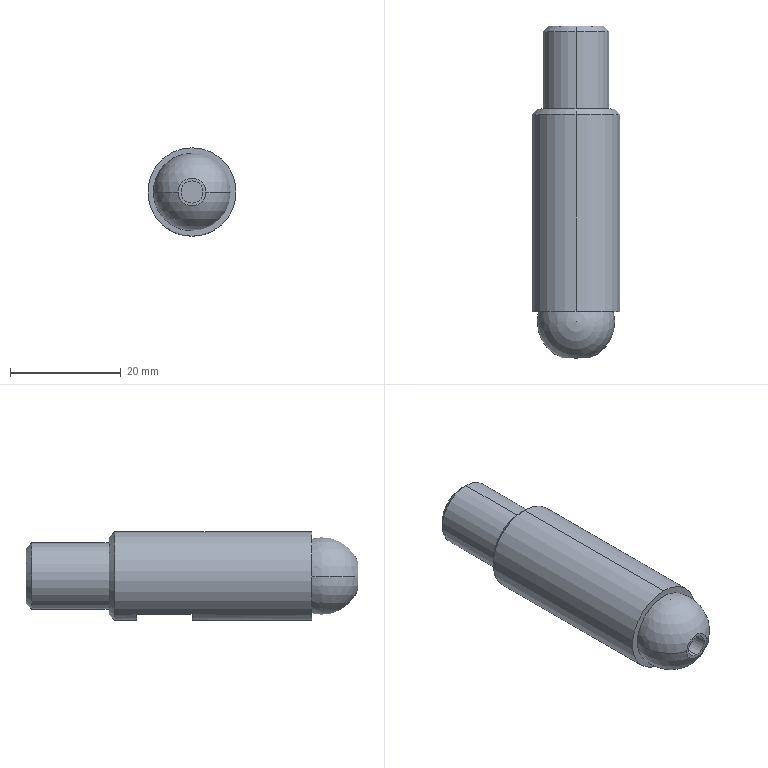Part | SolidWorks | features ICE 3, Chamfer 1, Revolution 1 | 1 solid | 24 faces | box 16 x 60 x 16 mm | volume 8216 mm3 | cylinder 9 | plane 9 | cone 4 | sphere 2 | commonest cylinder face diameters 12 x3 4 x2 8 x2 16 x2
STEP:
#1=CARTESIAN_POINT('',(0.,45.,7.));
#2=VERTEX_POINT('',#1);
#3=CARTESIAN_POINT('',(0.,45.,-7.));
#4=VERTEX_POINT('',#3);
#5=CARTESIAN_POINT('',(0.,45.,0.));
#6=DIRECTION('',(0.,1.,0.));
#7=DIRECTION('',(0.,0.,1.));
#8=AXIS2_PLACEMENT_3D('',#5,#6,#7);
#9=CIRCLE('',#8,7.);
#10=EDGE_CURVE('',#2,#4,#9,.T.);
#11=ORIENTED_EDGE('',*,*,#10,.F.);
#12=CARTESIAN_POINT('',(0.,44.,8.));
#13=VERTEX_POINT('',#12);
#14=CARTESIAN_POINT('',(0.,45.,7.));
#15=DIRECTION('',(0.,-0.7071,0.7071));
#16=VECTOR('',#15,1000.);
#17=LINE('',#14,#16);
#18=EDGE_CURVE('',#2,#13,#17,.T.);
#19=ORIENTED_EDGE('',*,*,#18,.T.);
#20=CARTESIAN_POINT('',(0.,44.,-8.));
#21=VERTEX_POINT('',#20);
#22=CARTESIAN_POINT('',(0.,44.,0.));
#23=DIRECTION('',(0.,-1.,0.));
#24=DIRECTION('',(0.,0.,1.));
#25=AXIS2_PLACEMENT_3D('',#22,#23,#24);
#26=CIRCLE('',#25,8.);
#27=EDGE_CURVE('',#21,#13,#26,.T.);
#28=ORIENTED_EDGE('',*,*,#27,.F.);
#29=CARTESIAN_POINT('',(0.,45.,-7.));
#30=DIRECTION('',(0.,-0.7071,-0.7071));
#31=VECTOR('',#30,1000.);
#32=LINE('',#29,#31);
#33=EDGE_CURVE('',#4,#21,#32,.T.);
#34=ORIENTED_EDGE('',*,*,#33,.F.);
#35=EDGE_LOOP('',(#11,#19,#28,#34));
#36=FACE_OUTER_BOUND('',#35,.T.);
#37=CARTESIAN_POINT('',(0.,45.,0.));
#38=DIRECTION('',(0.,-1.,0.));
#39=DIRECTION('',(0.,0.,-1.));
#40=AXIS2_PLACEMENT_3D('',#37,#38,#39);
#41=CONICAL_SURFACE('',#40,7.,0.7854);
#42=ADVANCED_FACE('',(#36),#41,.T.);
#43=CARTESIAN_POINT('',(0.,60.,5.));
#44=VERTEX_POINT('',#43);
#45=CARTESIAN_POINT('',(0.,60.,-5.));
#46=VERTEX_POINT('',#45);
#47=CARTESIAN_POINT('',(0.,60.,0.));
#48=DIRECTION('',(0.,1.,0.));
#49=DIRECTION('',(0.,0.,1.));
#50=AXIS2_PLACEMENT_3D('',#47,#48,#49);
#51=CIRCLE('',#50,5.);
#52=EDGE_CURVE('',#44,#46,#51,.T.);
#53=ORIENTED_EDGE('',*,*,#52,.F.);
#54=CARTESIAN_POINT('',(0.,59.,6.));
#55=VERTEX_POINT('',#54);
#56=CARTESIAN_POINT('',(0.,60.,5.));
#57=DIRECTION('',(0.,-0.7071,0.7071));
#58=VECTOR('',#57,1000.);
#59=LINE('',#56,#58);
#60=EDGE_CURVE('',#44,#55,#59,.T.);
#61=ORIENTED_EDGE('',*,*,#60,.T.);
#62=CARTESIAN_POINT('',(0.,59.,-6.));
#63=VERTEX_POINT('',#62);
#64=CARTESIAN_POINT('',(0.,59.,0.));
#65=DIRECTION('',(0.,-1.,0.));
#66=DIRECTION('',(0.,0.,1.));
#67=AXIS2_PLACEMENT_3D('',#64,#65,#66);
#68=CIRCLE('',#67,6.);
#69=EDGE_CURVE('',#63,#55,#68,.T.);
#70=ORIENTED_EDGE('',*,*,#69,.F.);
#71=CARTESIAN_POINT('',(0.,60.,-5.));
#72=DIRECTION('',(0.,-0.7071,-0.7071));
#73=VECTOR('',#72,1000.);
#74=LINE('',#71,#73);
#75=EDGE_CURVE('',#46,#63,#74,.T.);
#76=ORIENTED_EDGE('',*,*,#75,.F.);
#77=EDGE_LOOP('',(#53,#61,#70,#76));
#78=FACE_OUTER_BOUND('',#77,.T.);
#79=CARTESIAN_POINT('',(0.,60.,0.));
#80=DIRECTION('',(0.,-1.,0.));
#81=DIRECTION('',(0.,0.,-1.));
#82=AXIS2_PLACEMENT_3D('',#79,#80,#81);
#83=CONICAL_SURFACE('',#82,5.,0.7854);
#84=ADVANCED_FACE('',(#78),#83,.T.);
#85=ORIENTED_EDGE('',*,*,#69,.T.);
#86=CARTESIAN_POINT('',(0.,45.,6.));
#87=VERTEX_POINT('',#86);
#88=CARTESIAN_POINT('',(0.,60.,6.));
#89=DIRECTION('',(0.,-1.,0.));
#90=VECTOR('',#89,1000.);
#91=LINE('',#88,#90);
#92=EDGE_CURVE('',#55,#87,#91,.T.);
#93=ORIENTED_EDGE('',*,*,#92,.T.);
#94=CARTESIAN_POINT('',(0.,45.,-6.));
#95=VERTEX_POINT('',#94);
#96=CARTESIAN_POINT('',(0.,45.,0.));
#97=DIRECTION('',(0.,1.,0.));
#98=DIRECTION('',(0.,0.,1.));
#99=AXIS2_PLACEMENT_3D('',#96,#97,#98);
#100=CIRCLE('',#99,6.);
#101=EDGE_CURVE('',#87,#95,#100,.T.);
#102=ORIENTED_EDGE('',*,*,#101,.T.);
#103=CARTESIAN_POINT('',(0.,60.,-6.));
#104=DIRECTION('',(0.,-1.,0.));
#105=VECTOR('',#104,1000.);
#106=LINE('',#103,#105);
#107=EDGE_CURVE('',#63,#95,#106,.T.);
#108=ORIENTED_EDGE('',*,*,#107,.F.);
#109=EDGE_LOOP('',(#85,#93,#102,#108));
#110=FACE_OUTER_BOUND('',#109,.T.);
#111=CARTESIAN_POINT('',(0.,60.,0.));
#112=DIRECTION('',(0.,-1.,0.));
#113=DIRECTION('',(0.,0.,-1.));
#114=AXIS2_PLACEMENT_3D('',#111,#112,#113);
#115=CYLINDRICAL_SURFACE('',#114,6.);
#116=ADVANCED_FACE('',(#110),#115,.T.);
#117=ORIENTED_EDGE('',*,*,#27,.T.);
#118=CARTESIAN_POINT('',(0.,8.392,8.));
#119=VERTEX_POINT('',#118);
#120=CARTESIAN_POINT('',(0.,0.,8.));
#121=DIRECTION('',(0.,-1.,0.));
#122=VECTOR('',#121,1000.);
#123=LINE('',#120,#122);
#124=EDGE_CURVE('',#13,#119,#123,.T.);
#125=ORIENTED_EDGE('',*,*,#124,.T.);
#126=CARTESIAN_POINT('',(0.,8.392,-8.));
#127=VERTEX_POINT('',#126);
#128=CARTESIAN_POINT('',(0.,8.392,0.));
#129=DIRECTION('',(0.,-1.,0.));
#130=DIRECTION('',(0.,0.,-1.));
#131=AXIS2_PLACEMENT_3D('',#128,#129,#130);
#132=CIRCLE('',#131,8.);
#133=EDGE_CURVE('',#127,#119,#132,.T.);
#134=ORIENTED_EDGE('',*,*,#133,.F.);
#135=CARTESIAN_POINT('',(0.,30.,-8.));
#136=VERTEX_POINT('',#135);
#137=CARTESIAN_POINT('',(0.,0.,-8.));
#138=DIRECTION('',(0.,-1.,0.));
#139=VECTOR('',#138,1000.);
#140=LINE('',#137,#139);
#141=EDGE_CURVE('',#136,#127,#140,.T.);
#142=ORIENTED_EDGE('',*,*,#141,.F.);
#143=CARTESIAN_POINT('',(4.,30.,-6.928));
#144=VERTEX_POINT('',#143);
#145=CARTESIAN_POINT('',(0.,30.,0.));
#146=DIRECTION('',(0.,-1.,0.));
#147=DIRECTION('',(0.,0.,-1.));
#148=AXIS2_PLACEMENT_3D('',#145,#146,#147);
#149=CIRCLE('',#148,8.);
#150=EDGE_CURVE('',#136,#144,#149,.T.);
#151=ORIENTED_EDGE('',*,*,#150,.T.);
#152=CARTESIAN_POINT('',(4.,40.,-6.928));
#153=VERTEX_POINT('',#152);
#154=CARTESIAN_POINT('',(4.,40.,-6.928));
#155=DIRECTION('',(0.,-1.,0.));
#156=VECTOR('',#155,1000.);
#157=LINE('',#154,#156);
#158=EDGE_CURVE('',#153,#144,#157,.T.);
#159=ORIENTED_EDGE('',*,*,#158,.F.);
#160=CARTESIAN_POINT('',(0.,40.,-8.));
#161=VERTEX_POINT('',#160);
#162=CARTESIAN_POINT('',(0.,40.,0.));
#163=DIRECTION('',(0.,1.,0.));
#164=DIRECTION('',(0.,0.,1.));
#165=AXIS2_PLACEMENT_3D('',#162,#163,#164);
#166=CIRCLE('',#165,8.);
#167=EDGE_CURVE('',#153,#161,#166,.T.);
#168=ORIENTED_EDGE('',*,*,#167,.T.);
#169=CARTESIAN_POINT('',(0.,0.,-8.));
#170=DIRECTION('',(0.,-1.,0.));
#171=VECTOR('',#170,1000.);
#172=LINE('',#169,#171);
#173=EDGE_CURVE('',#21,#161,#172,.T.);
#174=ORIENTED_EDGE('',*,*,#173,.F.);
#175=EDGE_LOOP('',(#117,#125,#134,#142,#151,#159,#168,#174));
#176=FACE_OUTER_BOUND('',#175,.T.);
#177=CARTESIAN_POINT('',(0.,0.,0.));
#178=DIRECTION('',(0.,-1.,0.));
#179=DIRECTION('',(0.,0.,-1.));
#180=AXIS2_PLACEMENT_3D('',#177,#178,#179);
#181=CYLINDRICAL_SURFACE('',#180,8.);
#182=ADVANCED_FACE('',(#176),#181,.T.);
#183=CARTESIAN_POINT('',(0.,30.,4.));
#184=VERTEX_POINT('',#183);
#185=CARTESIAN_POINT('',(0.,30.,-4.));
#186=VERTEX_POINT('',#185);
#187=CARTESIAN_POINT('',(0.,30.,0.));
#188=DIRECTION('',(0.,-1.,0.));
#189=DIRECTION('',(0.,0.,-1.));
#190=AXIS2_PLACEMENT_3D('',#187,#188,#189);
#191=CIRCLE('',#190,4.);
#192=EDGE_CURVE('',#184,#186,#191,.T.);
#193=ORIENTED_EDGE('',*,*,#192,.F.);
#194=CARTESIAN_POINT('',(0.,27.,4.));
#195=VERTEX_POINT('',#194);
#196=CARTESIAN_POINT('',(0.,0.,4.));
#197=DIRECTION('',(0.,-1.,0.));
#198=VECTOR('',#197,1000.);
#199=LINE('',#196,#198);
#200=EDGE_CURVE('',#184,#195,#199,.T.);
#201=ORIENTED_EDGE('',*,*,#200,.T.);
#202=CARTESIAN_POINT('',(0.,27.,-4.));
#203=VERTEX_POINT('',#202);
#204=CARTESIAN_POINT('',(0.,27.,0.));
#205=DIRECTION('',(0.,-1.,0.));
#206=DIRECTION('',(0.,0.,-1.));
#207=AXIS2_PLACEMENT_3D('',#204,#205,#206);
#208=CIRCLE('',#207,4.);
#209=EDGE_CURVE('',#195,#203,#208,.T.);
#210=ORIENTED_EDGE('',*,*,#209,.T.);
#211=CARTESIAN_POINT('',(0.,0.,-4.));
#212=DIRECTION('',(0.,-1.,0.));
#213=VECTOR('',#212,1000.);
#214=LINE('',#211,#213);
#215=EDGE_CURVE('',#186,#203,#214,.T.);
#216=ORIENTED_EDGE('',*,*,#215,.F.);
#217=EDGE_LOOP('',(#193,#201,#210,#216));
#218=FACE_OUTER_BOUND('',#217,.T.);
#219=CARTESIAN_POINT('',(0.,0.,0.));
#220=DIRECTION('',(0.,-1.,0.));
#221=DIRECTION('',(0.,0.,-1.));
#222=AXIS2_PLACEMENT_3D('',#219,#220,#221);
#223=CYLINDRICAL_SURFACE('',#222,4.);
#224=ADVANCED_FACE('',(#218),#223,.F.);
#225=CARTESIAN_POINT('',(0.,27.,2.));
#226=VERTEX_POINT('',#225);
#227=CARTESIAN_POINT('',(0.,27.,-2.));
#228=VERTEX_POINT('',#227);
#229=CARTESIAN_POINT('',(0.,27.,0.));
#230=DIRECTION('',(0.,-1.,0.));
#231=DIRECTION('',(0.,0.,-1.));
#232=AXIS2_PLACEMENT_3D('',#229,#230,#231);
#233=CIRCLE('',#232,2.);
#234=EDGE_CURVE('',#226,#228,#233,.T.);
#235=ORIENTED_EDGE('',*,*,#234,.F.);
#236=CARTESIAN_POINT('',(0.,0.,2.));
#237=VERTEX_POINT('',#236);
#238=CARTESIAN_POINT('',(0.,0.,2.));
#239=DIRECTION('',(0.,-1.,0.));
#240=VECTOR('',#239,1000.);
#241=LINE('',#238,#240);
#242=EDGE_CURVE('',#226,#237,#241,.T.);
#243=ORIENTED_EDGE('',*,*,#242,.T.);
#244=CARTESIAN_POINT('',(0.,0.,-2.));
#245=VERTEX_POINT('',#244);
#246=CARTESIAN_POINT('',(0.,0.,0.));
#247=DIRECTION('',(0.,-1.,0.));
#248=DIRECTION('',(0.,0.,-1.));
#249=AXIS2_PLACEMENT_3D('',#246,#247,#248);
#250=CIRCLE('',#249,2.);
#251=EDGE_CURVE('',#237,#245,#250,.T.);
#252=ORIENTED_EDGE('',*,*,#251,.T.);
#253=CARTESIAN_POINT('',(0.,0.,-2.));
#254=DIRECTION('',(0.,-1.,0.));
#255=VECTOR('',#254,1000.);
#256=LINE('',#253,#255);
#257=EDGE_CURVE('',#228,#245,#256,.T.);
#258=ORIENTED_EDGE('',*,*,#257,.F.);
#259=EDGE_LOOP('',(#235,#243,#252,#258));
#260=FACE_OUTER_BOUND('',#259,.T.);
#261=CARTESIAN_POINT('',(0.,0.,0.));
#262=DIRECTION('',(0.,-1.,0.));
#263=DIRECTION('',(0.,0.,-1.));
#264=AXIS2_PLACEMENT_3D('',#261,#262,#263);
#265=CYLINDRICAL_SURFACE('',#264,2.);
#266=ADVANCED_FACE('',(#260),#265,.F.);
#267=CARTESIAN_POINT('',(-6.75,8.392,0.));
#268=VERTEX_POINT('',#267);
#269=CARTESIAN_POINT('',(6.75,8.392,0.));
#270=VERTEX_POINT('',#269);
#271=CARTESIAN_POINT('',(0.,8.392,0.));
#272=DIRECTION('',(0.,-1.,0.));
#273=DIRECTION('',(0.,0.,-1.));
#274=AXIS2_PLACEMENT_3D('',#271,#272,#273);
#275=CIRCLE('',#274,6.75);
#276=EDGE_CURVE('',#268,#270,#275,.T.);
#277=ORIENTED_EDGE('',*,*,#276,.T.);
#278=CARTESIAN_POINT('',(2.5,0.,0.));
#279=VERTEX_POINT('',#278);
#280=CARTESIAN_POINT('',(0.,6.538,0.));
#281=DIRECTION('',(0.,0.,-1.));
#282=DIRECTION('',(-1.,0.,0.));
#283=AXIS2_PLACEMENT_3D('',#280,#281,#282);
#284=CIRCLE('',#283,7.);
#285=EDGE_CURVE('',#270,#279,#284,.T.);
#286=ORIENTED_EDGE('',*,*,#285,.T.);
#287=CARTESIAN_POINT('',(-2.5,0.,0.));
#288=VERTEX_POINT('',#287);
#289=CARTESIAN_POINT('',(0.,0.,0.));
#290=DIRECTION('',(0.,-1.,0.));
#291=DIRECTION('',(0.,0.,-1.));
#292=AXIS2_PLACEMENT_3D('',#289,#290,#291);
#293=CIRCLE('',#292,2.5);
#294=EDGE_CURVE('',#288,#279,#293,.T.);
#295=ORIENTED_EDGE('',*,*,#294,.F.);
#296=CARTESIAN_POINT('',(0.,6.538,0.));
#297=DIRECTION('',(0.,0.,1.));
#298=DIRECTION('',(1.,0.,0.));
#299=AXIS2_PLACEMENT_3D('',#296,#297,#298);
#300=CIRCLE('',#299,7.);
#301=EDGE_CURVE('',#268,#288,#300,.T.);
#302=ORIENTED_EDGE('',*,*,#301,.F.);
#303=EDGE_LOOP('',(#277,#286,#295,#302));
#304=FACE_OUTER_BOUND('',#303,.T.);
#305=CARTESIAN_POINT('',(0.,6.538,0.));
#306=DIRECTION('',(0.,0.,-1.));
#307=DIRECTION('',(-1.,0.,0.));
#308=AXIS2_PLACEMENT_3D('',#305,#306,#307);
#309=SPHERICAL_SURFACE('',#308,7.);
#310=ADVANCED_FACE('',(#304),#309,.T.);
#311=CARTESIAN_POINT('',(0.,30.,0.));
#312=DIRECTION('',(0.,-1.,0.));
#313=DIRECTION('',(0.,0.,-1.));
#314=AXIS2_PLACEMENT_3D('',#311,#312,#313);
#315=CIRCLE('',#314,4.);
#316=EDGE_CURVE('',#186,#184,#315,.T.);
#317=ORIENTED_EDGE('',*,*,#316,.T.);
#318=ORIENTED_EDGE('',*,*,#192,.T.);
#319=EDGE_LOOP('',(#317,#318));
#320=FACE_BOUND('',#319,.T.);
#321=CARTESIAN_POINT('',(-4.,30.,-4.472));
#322=VERTEX_POINT('',#321);
#323=CARTESIAN_POINT('',(-4.,30.,-6.928));
#324=VERTEX_POINT('',#323);
#325=CARTESIAN_POINT('',(-4.,30.,-6.928));
#326=DIRECTION('',(0.,0.,-1.));
#327=VECTOR('',#326,1000.);
#328=LINE('',#325,#327);
#329=EDGE_CURVE('',#322,#324,#328,.T.);
#330=ORIENTED_EDGE('',*,*,#329,.F.);
#331=CARTESIAN_POINT('',(4.,30.,-4.472));
#332=VERTEX_POINT('',#331);
#333=CARTESIAN_POINT('',(0.,30.,0.));
#334=DIRECTION('',(0.,-1.,0.));
#335=DIRECTION('',(0.,0.,1.));
#336=AXIS2_PLACEMENT_3D('',#333,#334,#335);
#337=CIRCLE('',#336,6.);
#338=EDGE_CURVE('',#332,#322,#337,.T.);
#339=ORIENTED_EDGE('',*,*,#338,.F.);
#340=CARTESIAN_POINT('',(4.,30.,-4.472));
#341=DIRECTION('',(0.,0.,1.));
#342=VECTOR('',#341,1000.);
#343=LINE('',#340,#342);
#344=EDGE_CURVE('',#144,#332,#343,.T.);
#345=ORIENTED_EDGE('',*,*,#344,.F.);
#346=ORIENTED_EDGE('',*,*,#150,.F.);
#347=CARTESIAN_POINT('',(0.,30.,0.));
#348=DIRECTION('',(0.,-1.,0.));
#349=DIRECTION('',(0.,0.,-1.));
#350=AXIS2_PLACEMENT_3D('',#347,#348,#349);
#351=CIRCLE('',#350,8.);
#352=EDGE_CURVE('',#324,#136,#351,.T.);
#353=ORIENTED_EDGE('',*,*,#352,.F.);
#354=EDGE_LOOP('',(#330,#339,#345,#346,#353));
#355=FACE_OUTER_BOUND('',#354,.T.);
#356=CARTESIAN_POINT('',(-4.,30.,0.));
#357=DIRECTION('',(0.,-1.,0.));
#358=DIRECTION('',(0.,0.,-1.));
#359=AXIS2_PLACEMENT_3D('',#356,#357,#358);
#360=PLANE('',#359);
#361=ADVANCED_FACE('',(#320,#355),#360,.F.);
#362=ORIENTED_EDGE('',*,*,#285,.F.);
#363=CARTESIAN_POINT('',(0.,8.392,0.));
#364=DIRECTION('',(0.,-1.,0.));
#365=DIRECTION('',(0.,0.,-1.));
#366=AXIS2_PLACEMENT_3D('',#363,#364,#365);
#367=CIRCLE('',#366,6.75);
#368=EDGE_CURVE('',#270,#268,#367,.T.);
#369=ORIENTED_EDGE('',*,*,#368,.T.);
#370=ORIENTED_EDGE('',*,*,#301,.T.);
#371=CARTESIAN_POINT('',(0.,0.,0.));
#372=DIRECTION('',(0.,-1.,0.));
#373=DIRECTION('',(0.,0.,-1.));
#374=AXIS2_PLACEMENT_3D('',#371,#372,#373);
#375=CIRCLE('',#374,2.5);
#376=EDGE_CURVE('',#279,#288,#375,.T.);
#377=ORIENTED_EDGE('',*,*,#376,.F.);
#378=EDGE_LOOP('',(#362,#369,#370,#377));
#379=FACE_OUTER_BOUND('',#378,.T.);
#380=CARTESIAN_POINT('',(0.,6.538,0.));
#381=DIRECTION('',(0.,0.,-1.));
#382=DIRECTION('',(-1.,0.,0.));
#383=AXIS2_PLACEMENT_3D('',#380,#381,#382);
#384=SPHERICAL_SURFACE('',#383,7.);
#385=ADVANCED_FACE('',(#379),#384,.T.);
#386=CARTESIAN_POINT('',(0.,0.,0.));
#387=DIRECTION('',(0.,-1.,0.));
#388=DIRECTION('',(0.,0.,-1.));
#389=AXIS2_PLACEMENT_3D('',#386,#387,#388);
#390=CIRCLE('',#389,2.);
#391=EDGE_CURVE('',#245,#237,#390,.T.);
#392=ORIENTED_EDGE('',*,*,#391,.F.);
#393=ORIENTED_EDGE('',*,*,#251,.F.);
#394=EDGE_LOOP('',(#392,#393));
#395=FACE_BOUND('',#394,.T.);
#396=ORIENTED_EDGE('',*,*,#294,.T.);
#397=ORIENTED_EDGE('',*,*,#376,.T.);
#398=EDGE_LOOP('',(#396,#397));
#399=FACE_OUTER_BOUND('',#398,.T.);
#400=CARTESIAN_POINT('',(-2.,0.,0.));
#401=DIRECTION('',(0.,1.,0.));
#402=DIRECTION('',(0.,0.,1.));
#403=AXIS2_PLACEMENT_3D('',#400,#401,#402);
#404=PLANE('',#403);
#405=ADVANCED_FACE('',(#395,#399),#404,.F.);
#406=ORIENTED_EDGE('',*,*,#242,.F.);
#407=CARTESIAN_POINT('',(0.,27.,0.));
#408=DIRECTION('',(0.,-1.,0.));
#409=DIRECTION('',(0.,0.,-1.));
#410=AXIS2_PLACEMENT_3D('',#407,#408,#409);
#411=CIRCLE('',#410,2.);
#412=EDGE_CURVE('',#228,#226,#411,.T.);
#413=ORIENTED_EDGE('',*,*,#412,.F.);
#414=ORIENTED_EDGE('',*,*,#257,.T.);
#415=ORIENTED_EDGE('',*,*,#391,.T.);
#416=EDGE_LOOP('',(#406,#413,#414,#415));
#417=FACE_OUTER_BOUND('',#416,.T.);
#418=CARTESIAN_POINT('',(0.,0.,0.));
#419=DIRECTION('',(0.,-1.,0.));
#420=DIRECTION('',(0.,0.,-1.));
#421=AXIS2_PLACEMENT_3D('',#418,#419,#420);
#422=CYLINDRICAL_SURFACE('',#421,2.);
#423=ADVANCED_FACE('',(#417),#422,.F.);
#424=CARTESIAN_POINT('',(0.,27.,0.));
#425=DIRECTION('',(0.,-1.,0.));
#426=DIRECTION('',(0.,0.,-1.));
#427=AXIS2_PLACEMENT_3D('',#424,#425,#426);
#428=CIRCLE('',#427,4.);
#429=EDGE_CURVE('',#203,#195,#428,.T.);
#430=ORIENTED_EDGE('',*,*,#429,.F.);
#431=ORIENTED_EDGE('',*,*,#209,.F.);
#432=EDGE_LOOP('',(#430,#431));
#433=FACE_OUTER_BOUND('',#432,.T.);
#434=ORIENTED_EDGE('',*,*,#412,.T.);
#435=ORIENTED_EDGE('',*,*,#234,.T.);
#436=EDGE_LOOP('',(#434,#435));
#437=FACE_BOUND('',#436,.T.);
#438=CARTESIAN_POINT('',(-4.,27.,0.));
#439=DIRECTION('',(0.,-1.,0.));
#440=DIRECTION('',(0.,0.,-1.));
#441=AXIS2_PLACEMENT_3D('',#438,#439,#440);
#442=PLANE('',#441);
#443=ADVANCED_FACE('',(#433,#437),#442,.F.);
#444=ORIENTED_EDGE('',*,*,#200,.F.);
#445=ORIENTED_EDGE('',*,*,#316,.F.);
#446=ORIENTED_EDGE('',*,*,#215,.T.);
#447=ORIENTED_EDGE('',*,*,#429,.T.);
#448=EDGE_LOOP('',(#444,#445,#446,#447));
#449=FACE_OUTER_BOUND('',#448,.T.);
#450=CARTESIAN_POINT('',(0.,0.,0.));
#451=DIRECTION('',(0.,-1.,0.));
#452=DIRECTION('',(0.,0.,-1.));
#453=AXIS2_PLACEMENT_3D('',#450,#451,#452);
#454=CYLINDRICAL_SURFACE('',#453,4.);
#455=ADVANCED_FACE('',(#449),#454,.F.);
#456=ORIENTED_EDGE('',*,*,#124,.F.);
#457=CARTESIAN_POINT('',(0.,44.,0.));
#458=DIRECTION('',(0.,-1.,0.));
#459=DIRECTION('',(0.,0.,1.));
#460=AXIS2_PLACEMENT_3D('',#457,#458,#459);
#461=CIRCLE('',#460,8.);
#462=EDGE_CURVE('',#13,#21,#461,.T.);
#463=ORIENTED_EDGE('',*,*,#462,.T.);
#464=ORIENTED_EDGE('',*,*,#173,.T.);
#465=CARTESIAN_POINT('',(-4.,40.,-6.928));
#466=VERTEX_POINT('',#465);
#467=CARTESIAN_POINT('',(0.,40.,0.));
#468=DIRECTION('',(0.,1.,0.));
#469=DIRECTION('',(0.,0.,1.));
#470=AXIS2_PLACEMENT_3D('',#467,#468,#469);
#471=CIRCLE('',#470,8.);
#472=EDGE_CURVE('',#161,#466,#471,.T.);
#473=ORIENTED_EDGE('',*,*,#472,.T.);
#474=CARTESIAN_POINT('',(-4.,40.,-6.928));
#475=DIRECTION('',(0.,-1.,0.));
#476=VECTOR('',#475,1000.);
#477=LINE('',#474,#476);
#478=EDGE_CURVE('',#466,#324,#477,.T.);
#479=ORIENTED_EDGE('',*,*,#478,.T.);
#480=ORIENTED_EDGE('',*,*,#352,.T.);
#481=ORIENTED_EDGE('',*,*,#141,.T.);
#482=CARTESIAN_POINT('',(0.,8.392,0.));
#483=DIRECTION('',(0.,-1.,0.));
#484=DIRECTION('',(0.,0.,-1.));
#485=AXIS2_PLACEMENT_3D('',#482,#483,#484);
#486=CIRCLE('',#485,8.);
#487=EDGE_CURVE('',#119,#127,#486,.T.);
#488=ORIENTED_EDGE('',*,*,#487,.F.);
#489=EDGE_LOOP('',(#456,#463,#464,#473,#479,#480,#481,#488));
#490=FACE_OUTER_BOUND('',#489,.T.);
#491=CARTESIAN_POINT('',(0.,0.,0.));
#492=DIRECTION('',(0.,-1.,0.));
#493=DIRECTION('',(0.,0.,-1.));
#494=AXIS2_PLACEMENT_3D('',#491,#492,#493);
#495=CYLINDRICAL_SURFACE('',#494,8.);
#496=ADVANCED_FACE('',(#490),#495,.T.);
#497=ORIENTED_EDGE('',*,*,#276,.F.);
#498=ORIENTED_EDGE('',*,*,#368,.F.);
#499=EDGE_LOOP('',(#497,#498));
#500=FACE_BOUND('',#499,.T.);
#501=ORIENTED_EDGE('',*,*,#133,.T.);
#502=ORIENTED_EDGE('',*,*,#487,.T.);
#503=EDGE_LOOP('',(#501,#502));
#504=FACE_OUTER_BOUND('',#503,.T.);
#505=CARTESIAN_POINT('',(-8.,8.392,0.));
#506=DIRECTION('',(0.,1.,0.));
#507=DIRECTION('',(0.,0.,1.));
#508=AXIS2_PLACEMENT_3D('',#505,#506,#507);
#509=PLANE('',#508);
#510=ADVANCED_FACE('',(#500,#504),#509,.F.);
#511=ORIENTED_EDGE('',*,*,#344,.T.);
#512=CARTESIAN_POINT('',(4.,40.,-4.472));
#513=VERTEX_POINT('',#512);
#514=CARTESIAN_POINT('',(4.,40.,-4.472));
#515=DIRECTION('',(0.,-1.,0.));
#516=VECTOR('',#515,1000.);
#517=LINE('',#514,#516);
#518=EDGE_CURVE('',#513,#332,#517,.T.);
#519=ORIENTED_EDGE('',*,*,#518,.F.);
#520=CARTESIAN_POINT('',(4.,40.,-4.472));
#521=DIRECTION('',(0.,0.,1.));
#522=VECTOR('',#521,1000.);
#523=LINE('',#520,#522);
#524=EDGE_CURVE('',#153,#513,#523,.T.);
#525=ORIENTED_EDGE('',*,*,#524,.F.);
#526=ORIENTED_EDGE('',*,*,#158,.T.);
#527=EDGE_LOOP('',(#511,#519,#525,#526));
#528=FACE_OUTER_BOUND('',#527,.T.);
#529=CARTESIAN_POINT('',(4.,40.,-4.472));
#530=DIRECTION('',(1.,0.,0.));
#531=DIRECTION('',(0.,0.,-1.));
#532=AXIS2_PLACEMENT_3D('',#529,#530,#531);
#533=PLANE('',#532);
#534=ADVANCED_FACE('',(#528),#533,.F.);
#535=ORIENTED_EDGE('',*,*,#338,.T.);
#536=CARTESIAN_POINT('',(-4.,40.,-4.472));
#537=VERTEX_POINT('',#536);
#538=CARTESIAN_POINT('',(-4.,40.,-4.472));
#539=DIRECTION('',(0.,-1.,0.));
#540=VECTOR('',#539,1000.);
#541=LINE('',#538,#540);
#542=EDGE_CURVE('',#537,#322,#541,.T.);
#543=ORIENTED_EDGE('',*,*,#542,.F.);
#544=CARTESIAN_POINT('',(0.,40.,0.));
#545=DIRECTION('',(0.,-1.,0.));
#546=DIRECTION('',(0.,0.,1.));
#547=AXIS2_PLACEMENT_3D('',#544,#545,#546);
#548=CIRCLE('',#547,6.);
#549=EDGE_CURVE('',#513,#537,#548,.T.);
#550=ORIENTED_EDGE('',*,*,#549,.F.);
#551=ORIENTED_EDGE('',*,*,#518,.T.);
#552=EDGE_LOOP('',(#535,#543,#550,#551));
#553=FACE_OUTER_BOUND('',#552,.T.);
#554=CARTESIAN_POINT('',(0.,40.,0.));
#555=DIRECTION('',(0.,-1.,0.));
#556=DIRECTION('',(0.,0.,-1.));
#557=AXIS2_PLACEMENT_3D('',#554,#555,#556);
#558=CYLINDRICAL_SURFACE('',#557,6.);
#559=ADVANCED_FACE('',(#553),#558,.F.);
#560=ORIENTED_EDGE('',*,*,#329,.T.);
#561=ORIENTED_EDGE('',*,*,#478,.F.);
#562=CARTESIAN_POINT('',(-4.,40.,-6.928));
#563=DIRECTION('',(0.,0.,-1.));
#564=VECTOR('',#563,1000.);
#565=LINE('',#562,#564);
#566=EDGE_CURVE('',#537,#466,#565,.T.);
#567=ORIENTED_EDGE('',*,*,#566,.F.);
#568=ORIENTED_EDGE('',*,*,#542,.T.);
#569=EDGE_LOOP('',(#560,#561,#567,#568));
#570=FACE_OUTER_BOUND('',#569,.T.);
#571=CARTESIAN_POINT('',(-4.,40.,-6.928));
#572=DIRECTION('',(-1.,0.,0.));
#573=DIRECTION('',(0.,0.,1.));
#574=AXIS2_PLACEMENT_3D('',#571,#572,#573);
#575=PLANE('',#574);
#576=ADVANCED_FACE('',(#570),#575,.F.);
#577=ORIENTED_EDGE('',*,*,#167,.F.);
#578=ORIENTED_EDGE('',*,*,#524,.T.);
#579=ORIENTED_EDGE('',*,*,#549,.T.);
#580=ORIENTED_EDGE('',*,*,#566,.T.);
#581=ORIENTED_EDGE('',*,*,#472,.F.);
#582=EDGE_LOOP('',(#577,#578,#579,#580,#581));
#583=FACE_OUTER_BOUND('',#582,.T.);
#584=CARTESIAN_POINT('',(0.,40.,0.));
#585=DIRECTION('',(0.,1.,0.));
#586=DIRECTION('',(0.,0.,1.));
#587=AXIS2_PLACEMENT_3D('',#584,#585,#586);
#588=PLANE('',#587);
#589=ADVANCED_FACE('',(#583),#588,.F.);
#590=CARTESIAN_POINT('',(0.,45.,0.));
#591=DIRECTION('',(0.,1.,0.));
#592=DIRECTION('',(0.,0.,1.));
#593=AXIS2_PLACEMENT_3D('',#590,#591,#592);
#594=CIRCLE('',#593,7.);
#595=EDGE_CURVE('',#4,#2,#594,.T.);
#596=ORIENTED_EDGE('',*,*,#595,.T.);
#597=ORIENTED_EDGE('',*,*,#10,.T.);
#598=EDGE_LOOP('',(#596,#597));
#599=FACE_OUTER_BOUND('',#598,.T.);
#600=CARTESIAN_POINT('',(0.,45.,0.));
#601=DIRECTION('',(0.,1.,0.));
#602=DIRECTION('',(0.,0.,1.));
#603=AXIS2_PLACEMENT_3D('',#600,#601,#602);
#604=CIRCLE('',#603,6.);
#605=EDGE_CURVE('',#95,#87,#604,.T.);
#606=ORIENTED_EDGE('',*,*,#605,.F.);
#607=ORIENTED_EDGE('',*,*,#101,.F.);
#608=EDGE_LOOP('',(#606,#607));
#609=FACE_BOUND('',#608,.T.);
#610=CARTESIAN_POINT('',(0.,45.,0.));
#611=DIRECTION('',(0.,1.,0.));
#612=DIRECTION('',(0.,0.,1.));
#613=AXIS2_PLACEMENT_3D('',#610,#611,#612);
#614=PLANE('',#613);
#615=ADVANCED_FACE('',(#599,#609),#614,.T.);
#616=ORIENTED_EDGE('',*,*,#92,.F.);
#617=CARTESIAN_POINT('',(0.,59.,0.));
#618=DIRECTION('',(0.,-1.,0.));
#619=DIRECTION('',(0.,0.,1.));
#620=AXIS2_PLACEMENT_3D('',#617,#618,#619);
#621=CIRCLE('',#620,6.);
#622=EDGE_CURVE('',#55,#63,#621,.T.);
#623=ORIENTED_EDGE('',*,*,#622,.T.);
#624=ORIENTED_EDGE('',*,*,#107,.T.);
#625=ORIENTED_EDGE('',*,*,#605,.T.);
#626=EDGE_LOOP('',(#616,#623,#624,#625));
#627=FACE_OUTER_BOUND('',#626,.T.);
#628=CARTESIAN_POINT('',(0.,60.,0.));
#629=DIRECTION('',(0.,-1.,0.));
#630=DIRECTION('',(0.,0.,-1.));
#631=AXIS2_PLACEMENT_3D('',#628,#629,#630);
#632=CYLINDRICAL_SURFACE('',#631,6.);
#633=ADVANCED_FACE('',(#627),#632,.T.);
#634=CARTESIAN_POINT('',(0.,60.,0.));
#635=DIRECTION('',(0.,1.,0.));
#636=DIRECTION('',(0.,0.,1.));
#637=AXIS2_PLACEMENT_3D('',#634,#635,#636);
#638=CIRCLE('',#637,5.);
#639=EDGE_CURVE('',#46,#44,#638,.T.);
#640=ORIENTED_EDGE('',*,*,#639,.T.);
#641=ORIENTED_EDGE('',*,*,#52,.T.);
#642=EDGE_LOOP('',(#640,#641));
#643=FACE_OUTER_BOUND('',#642,.T.);
#644=CARTESIAN_POINT('',(0.,60.,0.));
#645=DIRECTION('',(0.,1.,0.));
#646=DIRECTION('',(0.,0.,1.));
#647=AXIS2_PLACEMENT_3D('',#644,#645,#646);
#648=PLANE('',#647);
#649=ADVANCED_FACE('',(#643),#648,.T.);
#650=ORIENTED_EDGE('',*,*,#60,.F.);
#651=ORIENTED_EDGE('',*,*,#639,.F.);
#652=ORIENTED_EDGE('',*,*,#75,.T.);
#653=ORIENTED_EDGE('',*,*,#622,.F.);
#654=EDGE_LOOP('',(#650,#651,#652,#653));
#655=FACE_OUTER_BOUND('',#654,.T.);
#656=CARTESIAN_POINT('',(0.,60.,0.));
#657=DIRECTION('',(0.,-1.,0.));
#658=DIRECTION('',(0.,0.,-1.));
#659=AXIS2_PLACEMENT_3D('',#656,#657,#658);
#660=CONICAL_SURFACE('',#659,5.,0.7854);
#661=ADVANCED_FACE('',(#655),#660,.T.);
#662=ORIENTED_EDGE('',*,*,#18,.F.);
#663=ORIENTED_EDGE('',*,*,#595,.F.);
#664=ORIENTED_EDGE('',*,*,#33,.T.);
#665=ORIENTED_EDGE('',*,*,#462,.F.);
#666=EDGE_LOOP('',(#662,#663,#664,#665));
#667=FACE_OUTER_BOUND('',#666,.T.);
#668=CARTESIAN_POINT('',(0.,45.,0.));
#669=DIRECTION('',(0.,-1.,0.));
#670=DIRECTION('',(0.,0.,-1.));
#671=AXIS2_PLACEMENT_3D('',#668,#669,#670);
#672=CONICAL_SURFACE('',#671,7.,0.7854);
#673=ADVANCED_FACE('',(#667),#672,.T.);
#674=CLOSED_SHELL('',(#42,#84,#116,#182,#224,#266,#310,#361,#385,#405,#423,#443,#455,#496,#510,#534,#559,#576,#589,#615,#633,#649,#661,#673));
#675=MANIFOLD_SOLID_BREP('',#674);
#676=CARTESIAN_POINT('',(0.,0.,0.));
#677=DIRECTION('',(0.,0.,1.));
#678=DIRECTION('',(1.,0.,0.));
#679=AXIS2_PLACEMENT_3D('',#676,#677,#678);
#680=(LENGTH_UNIT()NAMED_UNIT(*)SI_UNIT(.MILLI.,.METRE.));
#681=UNCERTAINTY_MEASURE_WITH_UNIT(LENGTH_MEASURE(0.00001),#680,'','');
#682=(NAMED_UNIT(*)PLANE_ANGLE_UNIT()SI_UNIT($,.RADIAN.));
#683=(NAMED_UNIT(*)SI_UNIT($,.STERADIAN.)SOLID_ANGLE_UNIT());
#684=(GEOMETRIC_REPRESENTATION_CONTEXT(3)GLOBAL_UNCERTAINTY_ASSIGNED_CONTEXT((#681))GLOBAL_UNIT_ASSIGNED_CONTEXT((#680,#682,#683))REPRESENTATION_CONTEXT('',''));
#685=ADVANCED_BREP_SHAPE_REPRESENTATION('',(#675,#679),#684);